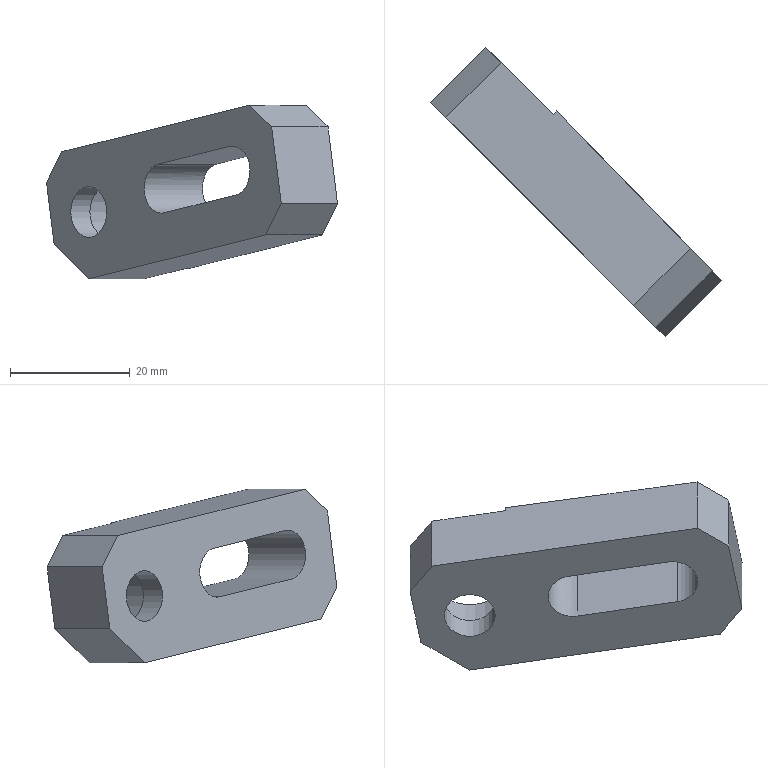Part | STEP file | gslz 2016.10.28-13_id1482_x_t | 1 solid | 19 faces | box 48.587 x 48.391 x 29.021 mm | volume 10993 mm3 | plane 10 | spline 7 | cylinder 2 | commonest cylinder face diameters 8.5 x1 14 x1